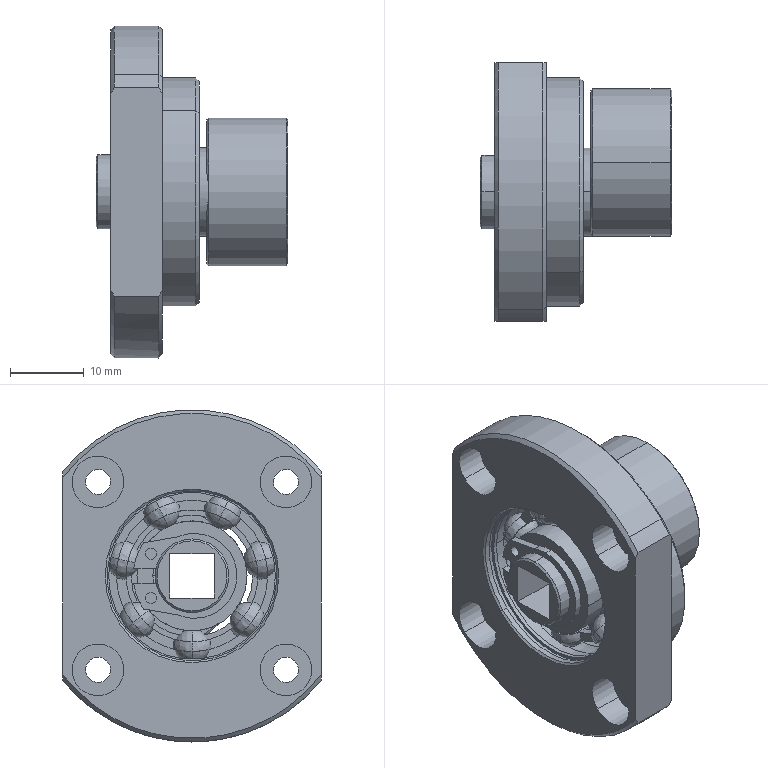Part | NX | features BREP 5 | 5 solids | 265 faces | box 26 x 35 x 45 mm | volume 12567 mm3 | cylinder 98 | sphere 56 | plane 54 | torus 32 | cone 25 | commonest cylinder face diameters 3.4 x8 7 x8 23.4 x8 10 x6 26 x6 1.5 x4